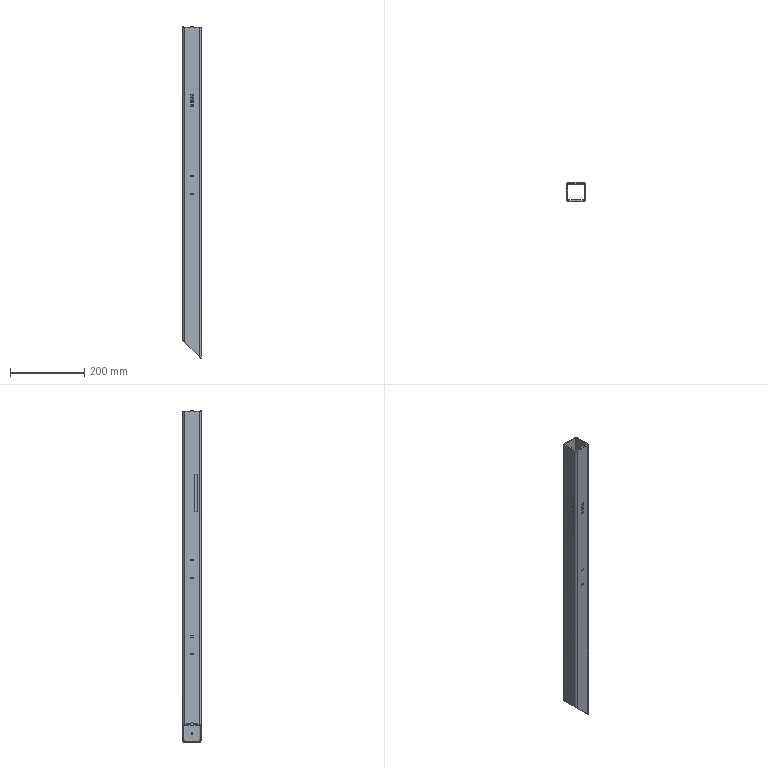Part | SolidWorks | features BaseBody 1 | 1 solid | 123 faces | box 50 x 50 x 893.5 mm | volume 465694 mm3 | plane 84 | cylinder 20 | spline 19 | commonest cylinder face diameters 4.2 x10 6 x4 12 x4 8 x2